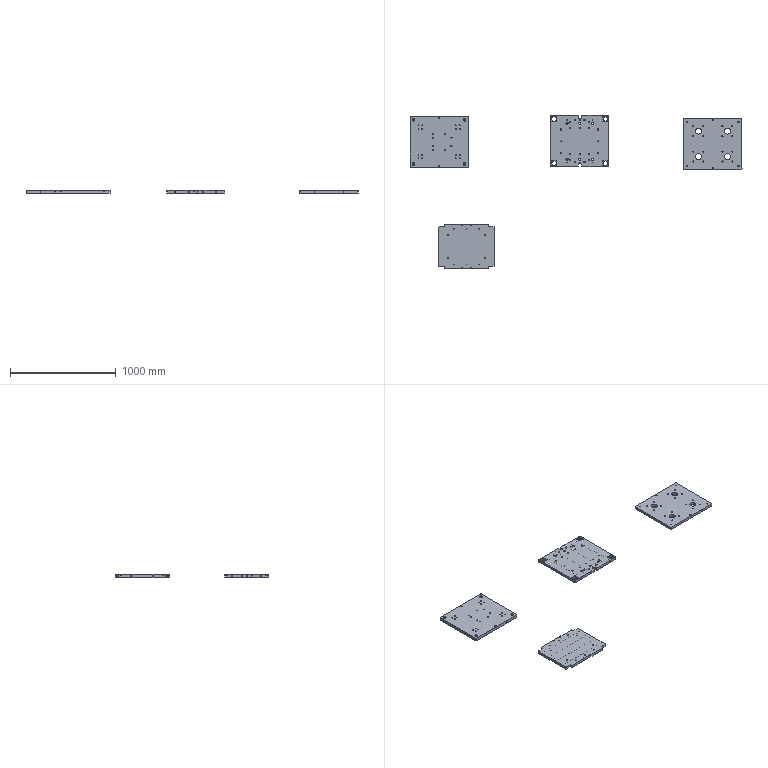NC program | Mastercam | posted with a generic post | part box 3140 x 1452 x 30 mm
Lines 1 to 2161 of 22248, first 1813 of 2161 lines:
%
O0000()
(MATERIAL - ALUMINUM MM - 2024)
( T16 | 16 FEM | H16 | XY STOCK TO LEAVE - .1 | Z STOCK TO LEAVE - .05 )
( T12 | 12 FEM | H12 | XY STOCK TO LEAVE - 0. | Z STOCK TO LEAVE - .05 )
( T7 | 4 CHM | H7 )
( T6 | 6 FEM | H6 | XY STOCK TO LEAVE - .05 | Z STOCK TO LEAVE - .15 )
( T15 | 5.2 DR | H15 | XY STOCK TO LEAVE - 0. | Z STOCK TO LEAVE - .15 )
( T3 | 10.5 DR | H3 )
( T19 | 9 DR | H19 )
N100 G21
N110 G0 G17 G40 G49 G80 G90
( ? )
N120 T16 M6
N130 G0 G90 G54 X-283.1 Y-255.5 A0. S6000 M3
N140 G43 H16 Z50. M8
N150 Z1.
N160 G1 Z-.499 F600.
N170 Y-237.5 F4000.
N180 Y237.5
N190 Y255.5
N200 Z-.998 F600.
N210 Y237.5 F4000.
N220 Y-237.5
N230 Y-255.5
N240 Z-1.497 F600.
N250 Y-237.5 F4000.
N260 Y237.5
N270 Y255.5
N280 Z-1.996 F600.
N290 Y237.5 F4000.
N300 Y-237.5
N310 Y-255.5
N320 Z-2.495 F600.
N330 Y-237.5 F4000.
N340 Y237.5
N350 Y255.5
N360 Z-2.994 F600.
N370 Y237.5 F4000.
N380 Y-237.5
N390 Y-255.5
N400 Z-3.493 F600.
N410 Y-237.5 F4000.
N420 Y237.5
N430 Y255.5
N440 Z-3.992 F600.
N450 Y237.5 F4000.
N460 Y-237.5
N470 Y-255.5
N480 Z-4.491 F600.
N490 Y-237.5 F4000.
N500 Y237.5
N510 Y255.5
N520 Z-4.99 F600.
N530 Y237.5 F4000.
N540 Y-237.5
N550 Y-255.5
N560 Z-5.489 F600.
N570 Y-237.5 F4000.
N580 Y237.5
N590 Y255.5
N600 Z-5.988 F600.
N610 Y237.5 F4000.
N620 Y-237.5
N630 Y-255.5
N640 Z-6.487 F600.
N650 Y-237.5 F4000.
N660 Y237.5
N670 Y255.5
N680 Z-6.986 F600.
N690 Y237.5 F4000.
N700 Y-237.5
N710 Y-255.5
N720 Z-7.485 F600.
N730 Y-237.5 F4000.
N740 Y237.5
N750 Y255.5
N760 Z-7.984 F600.
N770 Y237.5 F4000.
N780 Y-237.5
N790 Y-255.5
N800 Z-8.483 F600.
N810 Y-237.5 F4000.
N820 Y237.5
N830 Y255.5
N840 Z-8.982 F600.
N850 Y237.5 F4000.
N860 Y-237.5
N870 Y-255.5
N880 Z-9.481 F600.
N890 Y-237.5 F4000.
N900 Y237.5
N910 Y255.5
N920 Z-9.98 F600.
N930 Y237.5 F4000.
N940 Y-237.5
N950 Y-255.5
N960 Z-10.479 F600.
N970 Y-237.5 F4000.
N980 Y237.5
N990 Y255.5
N1000 Z-10.978 F600.
N1010 Y237.5 F4000.
N1020 Y-237.5
N1030 Y-255.5
N1040 Z-11.477 F600.
N1050 Y-237.5 F4000.
N1060 Y237.5
N1070 Y255.5
N1080 Z-11.976 F600.
N1090 Y237.5 F4000.
N1100 Y-237.5
N1110 Y-255.5
N1120 Z-12.475 F600.
N1130 Y-237.5 F4000.
N1140 Y237.5
N1150 Y255.5
N1160 Z-12.974 F600.
N1170 Y237.5 F4000.
N1180 Y-237.5
N1190 Y-255.5
N1200 Z-13.473 F600.
N1210 Y-237.5 F4000.
N1220 Y237.5
N1230 Y255.5
N1240 Z-13.972 F600.
N1250 Y237.5 F4000.
N1260 Y-237.5
N1270 Y-255.5
N1280 Z-14.471 F600.
N1290 Y-237.5 F4000.
N1300 Y237.5
N1310 Y255.5
N1320 Z-14.97 F600.
N1330 Y237.5 F4000.
N1340 Y-237.5
N1350 Y-255.5
N1360 Z-15.469 F600.
N1370 Y-237.5 F4000.
N1380 Y237.5
N1390 Y255.5
N1400 Z-15.968 F600.
N1410 Y237.5 F4000.
N1420 Y-237.5
N1430 Y-255.5
N1440 Z-16.467 F600.
N1450 Y-237.5 F4000.
N1460 Y237.5
N1470 Y255.5
N1480 Z-16.966 F600.
N1490 Y237.5 F4000.
N1500 Y-237.5
N1510 Y-255.5
N1520 Z-17.465 F600.
N1530 Y-237.5 F4000.
N1540 Y237.5
N1550 Y255.5
N1560 Z-17.964 F600.
N1570 Y237.5 F4000.
N1580 Y-237.5
N1590 Y-255.5
N1600 Z-18.463 F600.
N1610 Y-237.5 F4000.
N1620 Y237.5
N1630 Y255.5
N1640 Z-18.962 F600.
N1650 Y237.5 F4000.
N1660 Y-237.5
N1670 Y-255.5
N1680 Z-19.461 F600.
N1690 Y-237.5 F4000.
N1700 Y237.5
N1710 Y255.5
N1720 Z-19.96 F600.
N1730 Y237.5 F4000.
N1740 Y-237.5
N1750 Y-255.5
N1760 Z-20.459 F600.
N1770 Y-237.5 F4000.
N1780 Y237.5
N1790 Y255.5
N1800 Z-20.958 F600.
N1810 Y237.5 F4000.
N1820 Y-237.5
N1830 Y-255.5
N1840 Z-21.457 F600.
N1850 Y-237.5 F4000.
N1860 Y237.5
N1870 Y255.5
N1880 Z-21.956 F600.
N1890 Y237.5 F4000.
N1900 Y-237.5
N1910 Y-255.5
N1920 Z-22.455 F600.
N1930 Y-237.5 F4000.
N1940 Y237.5
N1950 Y255.5
N1960 Z-22.954 F600.
N1970 Y237.5 F4000.
N1980 Y-237.5
N1990 Y-255.5
N2000 Z-23.453 F600.
N2010 Y-237.5 F4000.
N2020 Y237.5
N2030 Y255.5
N2040 Z-23.952 F600.
N2050 Y237.5 F4000.
N2060 Y-237.5
N2070 Y-255.5
N2080 Z-24.451 F600.
N2090 Y-237.5 F4000.
N2100 Y237.5
N2110 Y255.5
N2120 Z-24.95 F600.
N2130 Y237.5 F4000.
N2140 Y-237.5
N2150 Y-255.5
N2160 G0 Z50.
N2170 X283.1 Y255.5
N2180 Z1.
N2190 G1 Z-.499 F600.
N2200 Y237.5 F4000.
N2210 Y-237.5
N2220 Y-255.5
N2230 Z-.998 F600.
N2240 Y-237.5 F4000.
N2250 Y237.5
N2260 Y255.5
N2270 Z-1.497 F600.
N2280 Y237.5 F4000.
N2290 Y-237.5
N2300 Y-255.5
N2310 Z-1.996 F600.
N2320 Y-237.5 F4000.
N2330 Y237.5
N2340 Y255.5
N2350 Z-2.495 F600.
N2360 Y237.5 F4000.
N2370 Y-237.5
N2380 Y-255.5
N2390 Z-2.994 F600.
N2400 Y-237.5 F4000.
N2410 Y237.5
N2420 Y255.5
N2430 Z-3.493 F600.
N2440 Y237.5 F4000.
N2450 Y-237.5
N2460 Y-255.5
N2470 Z-3.992 F600.
N2480 Y-237.5 F4000.
N2490 Y237.5
N2500 Y255.5
N2510 Z-4.491 F600.
N2520 Y237.5 F4000.
N2530 Y-237.5
N2540 Y-255.5
N2550 Z-4.99 F600.
N2560 Y-237.5 F4000.
N2570 Y237.5
N2580 Y255.5
N2590 Z-5.489 F600.
N2600 Y237.5 F4000.
N2610 Y-237.5
N2620 Y-255.5
N2630 Z-5.988 F600.
N2640 Y-237.5 F4000.
N2650 Y237.5
N2660 Y255.5
N2670 Z-6.487 F600.
N2680 Y237.5 F4000.
N2690 Y-237.5
N2700 Y-255.5
N2710 Z-6.986 F600.
N2720 Y-237.5 F4000.
N2730 Y237.5
N2740 Y255.5
N2750 Z-7.485 F600.
N2760 Y237.5 F4000.
N2770 Y-237.5
N2780 Y-255.5
N2790 Z-7.984 F600.
N2800 Y-237.5 F4000.
N2810 Y237.5
N2820 Y255.5
N2830 Z-8.483 F600.
N2840 Y237.5 F4000.
N2850 Y-237.5
N2860 Y-255.5
N2870 Z-8.982 F600.
N2880 Y-237.5 F4000.
N2890 Y237.5
N2900 Y255.5
N2910 Z-9.481 F600.
N2920 Y237.5 F4000.
N2930 Y-237.5
N2940 Y-255.5
N2950 Z-9.98 F600.
N2960 Y-237.5 F4000.
N2970 Y237.5
N2980 Y255.5
N2990 Z-10.479 F600.
N3000 Y237.5 F4000.
N3010 Y-237.5
N3020 Y-255.5
N3030 Z-10.978 F600.
N3040 Y-237.5 F4000.
N3050 Y237.5
N3060 Y255.5
N3070 Z-11.477 F600.
N3080 Y237.5 F4000.
N3090 Y-237.5
N3100 Y-255.5
N3110 Z-11.976 F600.
N3120 Y-237.5 F4000.
N3130 Y237.5
N3140 Y255.5
N3150 Z-12.475 F600.
N3160 Y237.5 F4000.
N3170 Y-237.5
N3180 Y-255.5
N3190 Z-12.974 F600.
N3200 Y-237.5 F4000.
N3210 Y237.5
N3220 Y255.5
N3230 Z-13.473 F600.
N3240 Y237.5 F4000.
N3250 Y-237.5
N3260 Y-255.5
N3270 Z-13.972 F600.
N3280 Y-237.5 F4000.
N3290 Y237.5
N3300 Y255.5
N3310 Z-14.471 F600.
N3320 Y237.5 F4000.
N3330 Y-237.5
N3340 Y-255.5
N3350 Z-14.97 F600.
N3360 Y-237.5 F4000.
N3370 Y237.5
N3380 Y255.5
N3390 Z-15.469 F600.
N3400 Y237.5 F4000.
N3410 Y-237.5
N3420 Y-255.5
N3430 Z-15.968 F600.
N3440 Y-237.5 F4000.
N3450 Y237.5
N3460 Y255.5
N3470 Z-16.467 F600.
N3480 Y237.5 F4000.
N3490 Y-237.5
N3500 Y-255.5
N3510 Z-16.966 F600.
N3520 Y-237.5 F4000.
N3530 Y237.5
N3540 Y255.5
N3550 Z-17.465 F600.
N3560 Y237.5 F4000.
N3570 Y-237.5
N3580 Y-255.5
N3590 Z-17.964 F600.
N3600 Y-237.5 F4000.
N3610 Y237.5
N3620 Y255.5
N3630 Z-18.463 F600.
N3640 Y237.5 F4000.
N3650 Y-237.5
N3660 Y-255.5
N3670 Z-18.962 F600.
N3680 Y-237.5 F4000.
N3690 Y237.5
N3700 Y255.5
N3710 Z-19.461 F600.
N3720 Y237.5 F4000.
N3730 Y-237.5
N3740 Y-255.5
N3750 Z-19.96 F600.
N3760 Y-237.5 F4000.
N3770 Y237.5
N3780 Y255.5
N3790 Z-20.459 F600.
N3800 Y237.5 F4000.
N3810 Y-237.5
N3820 Y-255.5
N3830 Z-20.958 F600.
N3840 Y-237.5 F4000.
N3850 Y237.5
N3860 Y255.5
N3870 Z-21.457 F600.
N3880 Y237.5 F4000.
N3890 Y-237.5
N3900 Y-255.5
N3910 Z-21.956 F600.
N3920 Y-237.5 F4000.
N3930 Y237.5
N3940 Y255.5
N3950 Z-22.455 F600.
N3960 Y237.5 F4000.
N3970 Y-237.5
N3980 Y-255.5
N3990 Z-22.954 F600.
N4000 Y-237.5 F4000.
N4010 Y237.5
N4020 Y255.5
N4030 Z-23.453 F600.
N4040 Y237.5 F4000.
N4050 Y-237.5
N4060 Y-255.5
N4070 Z-23.952 F600.
N4080 Y-237.5 F4000.
N4090 Y237.5
N4100 Y255.5
N4110 Z-24.451 F600.
N4120 Y237.5 F4000.
N4130 Y-237.5
N4140 Y-255.5
N4150 Z-24.95 F600.
N4160 Y-237.5 F4000.
N4170 Y237.5
N4180 Y255.5
N4190 G0 Z50.
N4200 M5
N4210 G91 G28 Z0. M9
N4220 A0.
N4230 M01
N4240 T12 M6
N4250 G0 G90 G17 G54 X-281. Y-255.5 A0. S6000 M3
N4260 G43 H12 Z50. M8
N4270 Z1.
N4280 G1 Z-12.475 F600.
N4290 Y-237.5 F1000.
N4300 Y237.5
N4310 Y255.5
N4320 G0 Z50.
N4330 Y-255.5
N4340 Z-11.475
N4350 G1 Z-24.95 F600.
N4360 Y-237.5 F1000.
N4370 Y237.5
N4380 Y255.5
N4390 G0 Z50.
N4400 X281.
N4410 Z1.
N4420 G1 Z-12.475 F600.
N4430 Y237.5 F1000.
N4440 Y-237.5
N4450 Y-255.5
N4460 G0 Z50.
N4470 Y255.5
N4480 Z-11.475
N4490 G1 Z-24.95 F600.
N4500 Y237.5 F1000.
N4510 Y-237.5
N4520 Y-255.5
N4530 G0 Z50.
N4540 M5
N4550 G91 G28 Z0. M9
N4560 A0.
N4570 M01
N4580 T7 M6
N4590 G0 G90 G17 G54 X-275.65 Y-242.5 A0. S6000 M3
N4600 G43 H7 Z50. M8
N4610 Z1.
N4620 G1 Z-.75 F600.
N4630 Y-237.5 F1000.
N4640 Y237.5
N4650 Y242.5
N4660 G0 Z50.
N4670 X275.65
N4680 Z1.
N4690 G1 Z-.75 F600.
N4700 Y237.5 F1000.
N4710 Y-237.5
N4720 Y-242.5
N4730 G0 Z50.
N4740 M5
N4750 G91 G28 Z0. M9
N4760 A0.
N4770 M01
( ?X )
M00
N4780 T16 M6
N4790 G0 G90 G17 G54 X-4. Y253.5 A0. S6000 M3
N4800 G43 H16 Z50. M8
N4810 Z1.
N4820 G1 Z-.693 F600.
N4830 Y237.5 F4000.
N4840 Y225.
N4850 G3 X0. Y221. I4. J0.
N4860 X4. Y225. I0. J4.
N4870 G1 Y237.5
N4880 Y253.5
N4890 Z-1.386 F600.
N4900 Y237.5 F4000.
N4910 Y225.
N4920 G2 X0. Y221. I-4. J0.
N4930 X-4. Y225. I0. J4.
N4940 G1 Y237.5
N4950 Y253.5
N4960 Z-2.079 F600.
N4970 Y237.5 F4000.
N4980 Y225.
N4990 G3 X0. Y221. I4. J0.
N5000 X4. Y225. I0. J4.
N5010 G1 Y237.5
N5020 Y253.5
N5030 Z-2.772 F600.
N5040 Y237.5 F4000.
N5050 Y225.
N5060 G2 X0. Y221. I-4. J0.
N5070 X-4. Y225. I0. J4.
N5080 G1 Y237.5
N5090 Y253.5
N5100 Z-3.465 F600.
N5110 Y237.5 F4000.
N5120 Y225.
N5130 G3 X0. Y221. I4. J0.
N5140 X4. Y225. I0. J4.
N5150 G1 Y237.5
N5160 Y253.5
N5170 Z-4.158 F600.
N5180 Y237.5 F4000.
N5190 Y225.
N5200 G2 X0. Y221. I-4. J0.
N5210 X-4. Y225. I0. J4.
N5220 G1 Y237.5
N5230 Y253.5
N5240 Z-4.851 F600.
N5250 Y237.5 F4000.
N5260 Y225.
N5270 G3 X0. Y221. I4. J0.
N5280 X4. Y225. I0. J4.
N5290 G1 Y237.5
N5300 Y253.5
N5310 Z-5.544 F600.
N5320 Y237.5 F4000.
N5330 Y225.
N5340 G2 X0. Y221. I-4. J0.
N5350 X-4. Y225. I0. J4.
N5360 G1 Y237.5
N5370 Y253.5
N5380 Z-6.237 F600.
N5390 Y237.5 F4000.
N5400 Y225.
N5410 G3 X0. Y221. I4. J0.
N5420 X4. Y225. I0. J4.
N5430 G1 Y237.5
N5440 Y253.5
N5450 Z-6.931 F600.
N5460 Y237.5 F4000.
N5470 Y225.
N5480 G2 X0. Y221. I-4. J0.
N5490 X-4. Y225. I0. J4.
N5500 G1 Y237.5
N5510 Y253.5
N5520 Z-7.624 F600.
N5530 Y237.5 F4000.
N5540 Y225.
N5550 G3 X0. Y221. I4. J0.
N5560 X4. Y225. I0. J4.
N5570 G1 Y237.5
N5580 Y253.5
N5590 Z-8.317 F600.
N5600 Y237.5 F4000.
N5610 Y225.
N5620 G2 X0. Y221. I-4. J0.
N5630 X-4. Y225. I0. J4.
N5640 G1 Y237.5
N5650 Y253.5
N5660 Z-9.01 F600.
N5670 Y237.5 F4000.
N5680 Y225.
N5690 G3 X0. Y221. I4. J0.
N5700 X4. Y225. I0. J4.
N5710 G1 Y237.5
N5720 Y253.5
N5730 Z-9.703 F600.
N5740 Y237.5 F4000.
N5750 Y225.
N5760 G2 X0. Y221. I-4. J0.
N5770 X-4. Y225. I0. J4.
N5780 G1 Y237.5
N5790 Y253.5
N5800 Z-10.396 F600.
N5810 Y237.5 F4000.
N5820 Y225.
N5830 G3 X0. Y221. I4. J0.
N5840 X4. Y225. I0. J4.
N5850 G1 Y237.5
N5860 Y253.5
N5870 Z-11.089 F600.
N5880 Y237.5 F4000.
N5890 Y225.
N5900 G2 X0. Y221. I-4. J0.
N5910 X-4. Y225. I0. J4.
N5920 G1 Y237.5
N5930 Y253.5
N5940 Z-11.782 F600.
N5950 Y237.5 F4000.
N5960 Y225.
N5970 G3 X0. Y221. I4. J0.
N5980 X4. Y225. I0. J4.
N5990 G1 Y237.5
N6000 Y253.5
N6010 Z-12.475 F600.
N6020 Y237.5 F4000.
N6030 Y225.
N6040 G2 X0. Y221. I-4. J0.
N6050 X-4. Y225. I0. J4.
N6060 G1 Y237.5
N6070 Y253.5
N6080 Z-13.168 F600.
N6090 Y237.5 F4000.
N6100 Y225.
N6110 G3 X0. Y221. I4. J0.
N6120 X4. Y225. I0. J4.
N6130 G1 Y237.5
N6140 Y253.5
N6150 Z-13.861 F600.
N6160 Y237.5 F4000.
N6170 Y225.
N6180 G2 X0. Y221. I-4. J0.
N6190 X-4. Y225. I0. J4.
N6200 G1 Y237.5
N6210 Y253.5
N6220 Z-14.554 F600.
N6230 Y237.5 F4000.
N6240 Y225.
N6250 G3 X0. Y221. I4. J0.
N6260 X4. Y225. I0. J4.
N6270 G1 Y237.5
N6280 Y253.5
N6290 Z-15.247 F600.
N6300 Y237.5 F4000.
N6310 Y225.
N6320 G2 X0. Y221. I-4. J0.
N6330 X-4. Y225. I0. J4.
N6340 G1 Y237.5
N6350 Y253.5
N6360 Z-15.94 F600.
N6370 Y237.5 F4000.
N6380 Y225.
N6390 G3 X0. Y221. I4. J0.
N6400 X4. Y225. I0. J4.
N6410 G1 Y237.5
N6420 Y253.5
N6430 Z-16.633 F600.
N6440 Y237.5 F4000.
N6450 Y225.
N6460 G2 X0. Y221. I-4. J0.
N6470 X-4. Y225. I0. J4.
N6480 G1 Y237.5
N6490 Y253.5
N6500 Z-17.326 F600.
N6510 Y237.5 F4000.
N6520 Y225.
N6530 G3 X0. Y221. I4. J0.
N6540 X4. Y225. I0. J4.
N6550 G1 Y237.5
N6560 Y253.5
N6570 Z-18.019 F600.
N6580 Y237.5 F4000.
N6590 Y225.
N6600 G2 X0. Y221. I-4. J0.
N6610 X-4. Y225. I0. J4.
N6620 G1 Y237.5
N6630 Y253.5
N6640 Z-18.712 F600.
N6650 Y237.5 F4000.
N6660 Y225.
N6670 G3 X0. Y221. I4. J0.
N6680 X4. Y225. I0. J4.
N6690 G1 Y237.5
N6700 Y253.5
N6710 Z-19.406 F600.
N6720 Y237.5 F4000.
N6730 Y225.
N6740 G2 X0. Y221. I-4. J0.
N6750 X-4. Y225. I0. J4.
N6760 G1 Y237.5
N6770 Y253.5
N6780 Z-20.099 F600.
N6790 Y237.5 F4000.
N6800 Y225.
N6810 G3 X0. Y221. I4. J0.
N6820 X4. Y225. I0. J4.
N6830 G1 Y237.5
N6840 Y253.5
N6850 Z-20.792 F600.
N6860 Y237.5 F4000.
N6870 Y225.
N6880 G2 X0. Y221. I-4. J0.
N6890 X-4. Y225. I0. J4.
N6900 G1 Y237.5
N6910 Y253.5
N6920 Z-21.485 F600.
N6930 Y237.5 F4000.
N6940 Y225.
N6950 G3 X0. Y221. I4. J0.
N6960 X4. Y225. I0. J4.
N6970 G1 Y237.5
N6980 Y253.5
N6990 Z-22.178 F600.
N7000 Y237.5 F4000.
N7010 Y225.
N7020 G2 X0. Y221. I-4. J0.
N7030 X-4. Y225. I0. J4.
N7040 G1 Y237.5
N7050 Y253.5
N7060 Z-22.871 F600.
N7070 Y237.5 F4000.
N7080 Y225.
N7090 G3 X0. Y221. I4. J0.
N7100 X4. Y225. I0. J4.
N7110 G1 Y237.5
N7120 Y253.5
N7130 Z-23.564 F600.
N7140 Y237.5 F4000.
N7150 Y225.
N7160 G2 X0. Y221. I-4. J0.
N7170 X-4. Y225. I0. J4.
N7180 G1 Y237.5
N7190 Y253.5
N7200 Z-24.257 F600.
N7210 Y237.5 F4000.
N7220 Y225.
N7230 G3 X0. Y221. I4. J0.
N7240 X4. Y225. I0. J4.
N7250 G1 Y237.5
N7260 Y253.5
N7270 Z-24.95 F600.
N7280 Y237.5 F4000.
N7290 Y225.
N7300 G2 X0. Y221. I-4. J0.
N7310 X-4. Y225. I0. J4.
N7320 G1 Y237.5
N7330 Y253.5
N7340 G0 Z50.
N7350 X4. Y-253.5
N7360 Z1.
N7370 G1 Z-.693 F600.
N7380 Y-237.5 F4000.
N7390 Y-225.
N7400 G3 X0. Y-221. I-4. J0.
N7410 X-4. Y-225. I0. J-4.
N7420 G1 Y-237.5
N7430 Y-253.5
N7440 Z-1.386 F600.
N7450 Y-237.5 F4000.
N7460 Y-225.
N7470 G2 X0. Y-221. I4. J0.
N7480 X4. Y-225. I0. J-4.
N7490 G1 Y-237.5
N7500 Y-253.5
N7510 Z-2.079 F600.
N7520 Y-237.5 F4000.
N7530 Y-225.
N7540 G3 X0. Y-221. I-4. J0.
N7550 X-4. Y-225. I0. J-4.
N7560 G1 Y-237.5
N7570 Y-253.5
N7580 Z-2.772 F600.
N7590 Y-237.5 F4000.
N7600 Y-225.
N7610 G2 X0. Y-221. I4. J0.
N7620 X4. Y-225. I0. J-4.
N7630 G1 Y-237.5
N7640 Y-253.5
N7650 Z-3.465 F600.
N7660 Y-237.5 F4000.
N7670 Y-225.
N7680 G3 X0. Y-221. I-4. J0.
N7690 X-4. Y-225. I0. J-4.
N7700 G1 Y-237.5
N7710 Y-253.5
N7720 Z-4.158 F600.
N7730 Y-237.5 F4000.
N7740 Y-225.
N7750 G2 X0. Y-221. I4. J0.
N7760 X4. Y-225. I0. J-4.
N7770 G1 Y-237.5
N7780 Y-253.5
N7790 Z-4.851 F600.
N7800 Y-237.5 F4000.
N7810 Y-225.
N7820 G3 X0. Y-221. I-4. J0.
N7830 X-4. Y-225. I0. J-4.
N7840 G1 Y-237.5
N7850 Y-253.5
N7860 Z-5.544 F600.
N7870 Y-237.5 F4000.
N7880 Y-225.
N7890 G2 X0. Y-221. I4. J0.
N7900 X4. Y-225. I0. J-4.
N7910 G1 Y-237.5
N7920 Y-253.5
N7930 Z-6.237 F600.
N7940 Y-237.5 F4000.
N7950 Y-225.
N7960 G3 X0. Y-221. I-4. J0.
N7970 X-4. Y-225. I0. J-4.
N7980 G1 Y-237.5
N7990 Y-253.5
N8000 Z-6.931 F600.
N8010 Y-237.5 F4000.
N8020 Y-225.
N8030 G2 X0. Y-221. I4. J0.
N8040 X4. Y-225. I0. J-4.
N8050 G1 Y-237.5
N8060 Y-253.5
N8070 Z-7.624 F600.
N8080 Y-237.5 F4000.
N8090 Y-225.
N8100 G3 X0. Y-221. I-4. J0.
N8110 X-4. Y-225. I0. J-4.
N8120 G1 Y-237.5
N8130 Y-253.5
N8140 Z-8.317 F600.
N8150 Y-237.5 F4000.
N8160 Y-225.
N8170 G2 X0. Y-221. I4. J0.
N8180 X4. Y-225. I0. J-4.
N8190 G1 Y-237.5
N8200 Y-253.5
N8210 Z-9.01 F600.
N8220 Y-237.5 F4000.
N8230 Y-225.
N8240 G3 X0. Y-221. I-4. J0.
N8250 X-4. Y-225. I0. J-4.
N8260 G1 Y-237.5
N8270 Y-253.5
N8280 Z-9.703 F600.
N8290 Y-237.5 F4000.
N8300 Y-225.
N8310 G2 X0. Y-221. I4. J0.
N8320 X4. Y-225. I0. J-4.
N8330 G1 Y-237.5
N8340 Y-253.5
N8350 Z-10.396 F600.
N8360 Y-237.5 F4000.
N8370 Y-225.
N8380 G3 X0. Y-221. I-4. J0.
N8390 X-4. Y-225. I0. J-4.
N8400 G1 Y-237.5
N8410 Y-253.5
N8420 Z-11.089 F600.
N8430 Y-237.5 F4000.
N8440 Y-225.
N8450 G2 X0. Y-221. I4. J0.
N8460 X4. Y-225. I0. J-4.
N8470 G1 Y-237.5
N8480 Y-253.5
N8490 Z-11.782 F600.
N8500 Y-237.5 F4000.
N8510 Y-225.
N8520 G3 X0. Y-221. I-4. J0.
N8530 X-4. Y-225. I0. J-4.
N8540 G1 Y-237.5
N8550 Y-253.5
N8560 Z-12.475 F600.
N8570 Y-237.5 F4000.
N8580 Y-225.
N8590 G2 X0. Y-221. I4. J0.
N8600 X4. Y-225. I0. J-4.
N8610 G1 Y-237.5
N8620 Y-253.5
N8630 Z-13.168 F600.
N8640 Y-237.5 F4000.
N8650 Y-225.
N8660 G3 X0. Y-221. I-4. J0.
N8670 X-4. Y-225. I0. J-4.
N8680 G1 Y-237.5
N8690 Y-253.5
N8700 Z-13.861 F600.
N8710 Y-237.5 F4000.
N8720 Y-225.
N8730 G2 X0. Y-221. I4. J0.
N8740 X4. Y-225. I0. J-4.
N8750 G1 Y-237.5
N8760 Y-253.5
N8770 Z-14.554 F600.
N8780 Y-237.5 F4000.
N8790 Y-225.
N8800 G3 X0. Y-221. I-4. J0.
N8810 X-4. Y-225. I0. J-4.
N8820 G1 Y-237.5
N8830 Y-253.5
N8840 Z-15.247 F600.
N8850 Y-237.5 F4000.
N8860 Y-225.
N8870 G2 X0. Y-221. I4. J0.
N8880 X4. Y-225. I0. J-4.
N8890 G1 Y-237.5
N8900 Y-253.5
N8910 Z-15.94 F600.
N8920 Y-237.5 F4000.
N8930 Y-225.
N8940 G3 X0. Y-221. I-4. J0.
N8950 X-4. Y-225. I0. J-4.
N8960 G1 Y-237.5
N8970 Y-253.5
N8980 Z-16.633 F600.
N8990 Y-237.5 F4000.
N9000 Y-225.
N9010 G2 X0. Y-221. I4. J0.
N9020 X4. Y-225. I0. J-4.
N9030 G1 Y-237.5
N9040 Y-253.5
N9050 Z-17.326 F600.
N9060 Y-237.5 F4000.
N9070 Y-225.
N9080 G3 X0. Y-221. I-4. J0.
N9090 X-4. Y-225. I0. J-4.
N9100 G1 Y-237.5
N9110 Y-253.5
N9120 Z-18.019 F600.
N9130 Y-237.5 F4000.
N9140 Y-225.
N9150 G2 X0. Y-221. I4. J0.
N9160 X4. Y-225. I0. J-4.
N9170 G1 Y-237.5
N9180 Y-253.5
N9190 Z-18.712 F600.
N9200 Y-237.5 F4000.
N9210 Y-225.
N9220 G3 X0. Y-221. I-4. J0.
N9230 X-4. Y-225. I0. J-4.
N9240 G1 Y-237.5
N9250 Y-253.5
N9260 Z-19.406 F600.
N9270 Y-237.5 F4000.
N9280 Y-225.
N9290 G2 X0. Y-221. I4. J0.
N9300 X4. Y-225. I0. J-4.
N9310 G1 Y-237.5
N9320 Y-253.5
N9330 Z-20.099 F600.
N9340 Y-237.5 F4000.
N9350 Y-225.
N9360 G3 X0. Y-221. I-4. J0.
N9370 X-4. Y-225. I0. J-4.
N9380 G1 Y-237.5
N9390 Y-253.5
N9400 Z-20.792 F600.
N9410 Y-237.5 F4000.
N9420 Y-225.
N9430 G2 X0. Y-221. I4. J0.
N9440 X4. Y-225. I0. J-4.
N9450 G1 Y-237.5
N9460 Y-253.5
N9470 Z-21.485 F600.
N9480 Y-237.5 F4000.
N9490 Y-225.
N9500 G3 X0. Y-221. I-4. J0.
N9510 X-4. Y-225. I0. J-4.
N9520 G1 Y-237.5
N9530 Y-253.5
N9540 Z-22.178 F600.
N9550 Y-237.5 F4000.
N9560 Y-225.
N9570 G2 X0. Y-221. I4. J0.
N9580 X4. Y-225. I0. J-4.
N9590 G1 Y-237.5
N9600 Y-253.5
N9610 Z-22.871 F600.
N9620 Y-237.5 F4000.
N9630 Y-225.
N9640 G3 X0. Y-221. I-4. J0.
N9650 X-4. Y-225. I0. J-4.
N9660 G1 Y-237.5
N9670 Y-253.5
N9680 Z-23.564 F600.
N9690 Y-237.5 F4000.
N9700 Y-225.
N9710 G2 X0. Y-221. I4. J0.
N9720 X4. Y-225. I0. J-4.
N9730 G1 Y-237.5
N9740 Y-253.5
N9750 Z-24.257 F600.
N9760 Y-237.5 F4000.
N9770 Y-225.
N9780 G3 X0. Y-221. I-4. J0.
N9790 X-4. Y-225. I0. J-4.
N9800 G1 Y-237.5
N9810 Y-253.5
N9820 Z-24.95 F600.
N9830 Y-237.5 F4000.
N9840 Y-225.
N9850 G2 X0. Y-221. I4. J0.
N9860 X4. Y-225. I0. J-4.
N9870 G1 Y-237.5
N9880 Y-253.5
N9890 G0 Z50.
N9900 X286.3 Y-235.9
N9910 Z1.
N9920 G1 Z-.693 F600.
N9930 X284.7 F4000.
N9940 G3 X283.1 Y-237.5 I0. J-1.6
N9950 G2 X270. Y-250.6 I-13.1 J0.
N9960 G1 X20.
N9970 G2 X6.9 Y-237.5 I0. J13.1
N9980 G1 Y-225.
N9990 G3 X0. Y-218.1 I-6.9 J0.
N100 X-6.9 Y-225. I0. J-6.9
N110 G1 Y-237.5
N120 G2 X-20. Y-250.6 I-13.1 J0.
N130 G1 X-270.
N140 G2 X-283.1 Y-237.5 I0. J13.1
N150 G3 X-284.7 Y-235.9 I-1.6 J0.
N160 G1 X-286.3
N170 Z-1.386 F600.
N180 X-284.7 F4000.
N190 G2 X-283.1 Y-237.5 I0. J-1.6
N200 G3 X-270. Y-250.6 I13.1 J0.
N210 G1 X-20.
N220 G3 X-6.9 Y-237.5 I0. J13.1
N230 G1 Y-225.
N240 G2 X0. Y-218.1 I6.9 J0.
N250 X6.9 Y-225. I0. J-6.9
N260 G1 Y-237.5
N270 G3 X20. Y-250.6 I13.1 J0.
N280 G1 X270.
N290 G3 X283.1 Y-237.5 I0. J13.1
N300 G2 X284.7 Y-235.9 I1.6 J0.
N310 G1 X286.3
N320 Z-2.079 F600.
N330 X284.7 F4000.
N340 G3 X283.1 Y-237.5 I0. J-1.6
N350 G2 X270. Y-250.6 I-13.1 J0.
N360 G1 X20.
N370 G2 X6.9 Y-237.5 I0. J13.1
N380 G1 Y-225.
N390 G3 X0. Y-218.1 I-6.9 J0.
N400 X-6.9 Y-225. I0. J-6.9
N410 G1 Y-237.5
N420 G2 X-20. Y-250.6 I-13.1 J0.
N430 G1 X-270.
N440 G2 X-283.1 Y-237.5 I0. J13.1
N450 G3 X-284.7 Y-235.9 I-1.6 J0.
N460 G1 X-286.3
N470 Z-2.772 F600.
N480 X-284.7 F4000.
N490 G2 X-283.1 Y-237.5 I0. J-1.6
N500 G3 X-270. Y-250.6 I13.1 J0.
N510 G1 X-20.
N520 G3 X-6.9 Y-237.5 I0. J13.1
N530 G1 Y-225.
N540 G2 X0. Y-218.1 I6.9 J0.
N550 X6.9 Y-225. I0. J-6.9
N560 G1 Y-237.5
N570 G3 X20. Y-250.6 I13.1 J0.
N580 G1 X270.
N590 G3 X283.1 Y-237.5 I0. J13.1
N600 G2 X284.7 Y-235.9 I1.6 J0.
N610 G1 X286.3
N620 Z-3.465 F600.
N630 X284.7 F4000.
N640 G3 X283.1 Y-237.5 I0. J-1.6
N650 G2 X270. Y-250.6 I-13.1 J0.
N660 G1 X20.
N670 G2 X6.9 Y-237.5 I0. J13.1
N680 G1 Y-225.
N690 G3 X0. Y-218.1 I-6.9 J0.
N700 X-6.9 Y-225. I0. J-6.9
N710 G1 Y-237.5
N720 G2 X-20. Y-250.6 I-13.1 J0.
N730 G1 X-270.
N740 G2 X-283.1 Y-237.5 I0. J13.1
N750 G3 X-284.7 Y-235.9 I-1.6 J0.
N760 G1 X-286.3
N770 Z-4.158 F600.
N780 X-284.7 F4000.
N790 G2 X-283.1 Y-237.5 I0. J-1.6
N800 G3 X-270. Y-250.6 I13.1 J0.
N810 G1 X-20.
N820 G3 X-6.9 Y-237.5 I0. J13.1
N830 G1 Y-225.
N840 G2 X0. Y-218.1 I6.9 J0.
N850 X6.9 Y-225. I0. J-6.9
N860 G1 Y-237.5
N870 G3 X20. Y-250.6 I13.1 J0.
N880 G1 X270.
N890 G3 X283.1 Y-237.5 I0. J13.1
N900 G2 X284.7 Y-235.9 I1.6 J0.
N910 G1 X286.3
N920 Z-4.851 F600.
N930 X284.7 F4000.
N940 G3 X283.1 Y-237.5 I0. J-1.6
N950 G2 X270. Y-250.6 I-13.1 J0.
N960 G1 X20.
N970 G2 X6.9 Y-237.5 I0. J13.1
N980 G1 Y-225.
N990 G3 X0. Y-218.1 I-6.9 J0.
N1000 X-6.9 Y-225. I0. J-6.9
N1010 G1 Y-237.5
N1020 G2 X-20. Y-250.6 I-13.1 J0.
N1030 G1 X-270.
N1040 G2 X-283.1 Y-237.5 I0. J13.1
N1050 G3 X-284.7 Y-235.9 I-1.6 J0.
N1060 G1 X-286.3
N1070 Z-5.544 F600.
N1080 X-284.7 F4000.
N1090 G2 X-283.1 Y-237.5 I0. J-1.6
N1100 G3 X-270. Y-250.6 I13.1 J0.
N1110 G1 X-20.
N1120 G3 X-6.9 Y-237.5 I0. J13.1
N1130 G1 Y-225.
N1140 G2 X0. Y-218.1 I6.9 J0.
N1150 X6.9 Y-225. I0. J-6.9
N1160 G1 Y-237.5
N1170 G3 X20. Y-250.6 I13.1 J0.
N1180 G1 X270.
N1190 G3 X283.1 Y-237.5 I0. J13.1
N1200 G2 X284.7 Y-235.9 I1.6 J0.
N1210 G1 X286.3
N1220 Z-6.237 F600.
N1230 X284.7 F4000.
N1240 G3 X283.1 Y-237.5 I0. J-1.6
N1250 G2 X270. Y-250.6 I-13.1 J0.
N1260 G1 X20.
N1270 G2 X6.9 Y-237.5 I0. J13.1
N1280 G1 Y-225.
N1290 G3 X0. Y-218.1 I-6.9 J0.
N1300 X-6.9 Y-225. I0. J-6.9
N1310 G1 Y-237.5
N1320 G2 X-20. Y-250.6 I-13.1 J0.
N1330 G1 X-270.
N1340 G2 X-283.1 Y-237.5 I0. J13.1
N1350 G3 X-284.7 Y-235.9 I-1.6 J0.
N1360 G1 X-286.3
N1370 Z-6.931 F600.
N1380 X-284.7 F4000.
N1390 G2 X-283.1 Y-237.5 I0. J-1.6
N1400 G3 X-270. Y-250.6 I13.1 J0.
N1410 G1 X-20.
N1420 G3 X-6.9 Y-237.5 I0. J13.1
N1430 G1 Y-225.
N1440 G2 X0. Y-218.1 I6.9 J0.
N1450 X6.9 Y-225. I0. J-6.9
N1460 G1 Y-237.5
N1470 G3 X20. Y-250.6 I13.1 J0.
N1480 G1 X270.
N1490 G3 X283.1 Y-237.5 I0. J13.1
N1500 G2 X284.7 Y-235.9 I1.6 J0.
N1510 G1 X286.3
N1520 Z-7.624 F600.
N1530 X284.7 F4000.
N1540 G3 X283.1 Y-237.5 I0. J-1.6
N1550 G2 X270. Y-250.6 I-13.1 J0.
N1560 G1 X20.
N1570 G2 X6.9 Y-237.5 I0. J13.1
N1580 G1 Y-225.
N1590 G3 X0. Y-218.1 I-6.9 J0.
N1600 X-6.9 Y-225. I0. J-6.9
N1610 G1 Y-237.5
N1620 G2 X-20. Y-250.6 I-13.1 J0.
N1630 G1 X-270.
N1640 G2 X-283.1 Y-237.5 I0. J13.1
N1650 G3 X-284.7 Y-235.9 I-1.6 J0.
N1660 G1 X-286.3
N1670 Z-8.317 F600.
N1680 X-284.7 F4000.
N1690 G2 X-283.1 Y-237.5 I0. J-1.6
N1700 G3 X-270. Y-250.6 I13.1 J0.
N1710 G1 X-20.
N1720 G3 X-6.9 Y-237.5 I0. J13.1
N1730 G1 Y-225.
N1740 G2 X0. Y-218.1 I6.9 J0.
N1750 X6.9 Y-225. I0. J-6.9
N1760 G1 Y-237.5
N1770 G3 X20. Y-250.6 I13.1 J0.
N1780 G1 X270.
N1790 G3 X283.1 Y-237.5 I0. J13.1
N1800 G2 X284.7 Y-235.9 I1.6 J0.
N1810 G1 X286.3
N1820 Z-9.01 F600.
N1830 X284.7 F4000.
N1840 G3 X283.1 Y-237.5 I0. J-1.6
N1850 G2 X270. Y-250.6 I-13.1 J0.
N1860 G1 X20.
N1870 G2 X6.9 Y-237.5 I0. J13.1
N1880 G1 Y-225.
N1890 G3 X0. Y-218.1 I-6.9 J0.
N1900 X-6.9 Y-225. I0. J-6.9
N1910 G1 Y-237.5
N1920 G2 X-20. Y-250.6 I-13.1 J0.
N1930 G1 X-270.
N1940 G2 X-283.1 Y-237.5 I0. J13.1
N1950 G3 X-284.7 Y-235.9 I-1.6 J0.
N1960 G1 X-286.3
N1970 Z-9.703 F600.
N1980 X-284.7 F4000.
N1990 G2 X-283.1 Y-237.5 I0. J-1.6
N2000 G3 X-270. Y-250.6 I13.1 J0.
N2010 G1 X-20.
N2020 G3 X-6.9 Y-237.5 I0. J13.1
N2030 G1 Y-225.
N2040 G2 X0. Y-218.1 I6.9 J0.
N2050 X6.9 Y-225. I0. J-6.9
N2060 G1 Y-237.5
N2070 G3 X20. Y-250.6 I13.1 J0.
N2080 G1 X270.
N2090 G3 X283.1 Y-237.5 I0. J13.1
N2100 G2 X284.7 Y-235.9 I1.6 J0.
N2110 G1 X286.3
N2120 Z-10.396 F600.
N2130 X284.7 F4000.
N2140 G3 X283.1 Y-237.5 I0. J-1.6
N2150 G2 X270. Y-250.6 I-13.1 J0.
N2160 G1 X20.
N2170 G2 X6.9 Y-237.5 I0. J13.1
N2180 G1 Y-225.
N2190 G3 X0. Y-218.1 I-6.9 J0.
N2200 X-6.9 Y-225. I0. J-6.9
N2210 G1 Y-237.5
N2220 G2 X-20. Y-250.6 I-13.1 J0.
N2230 G1 X-270.
N2240 G2 X-283.1 Y-237.5 I0. J13.1
N2250 G3 X-284.7 Y-235.9 I-1.6 J0.
N2260 G1 X-286.3
N2270 Z-11.089 F600.
N2280 X-284.7 F4000.
N2290 G2 X-283.1 Y-237.5 I0. J-1.6
N2300 G3 X-270. Y-250.6 I13.1 J0.
N2310 G1 X-20.
N2320 G3 X-6.9 Y-237.5 I0. J13.1
N2330 G1 Y-225.
N2340 G2 X0. Y-218.1 I6.9 J0.
N2350 X6.9 Y-225. I0. J-6.9
N2360 G1 Y-237.5
N2370 G3 X20. Y-250.6 I13.1 J0.
N2380 G1 X270.
N2390 G3 X283.1 Y-237.5 I0. J13.1
N2400 G2 X284.7 Y-235.9 I1.6 J0.
N2410 G1 X286.3
N2420 Z-11.782 F600.
N2430 X284.7 F4000.
N2440 G3 X283.1 Y-237.5 I0. J-1.6
N2450 G2 X270. Y-250.6 I-13.1 J0.
N2460 G1 X20.
N2470 G2 X6.9 Y-237.5 I0. J13.1
N2480 G1 Y-225.
N2490 G3 X0. Y-218.1 I-6.9 J0.
N2500 X-6.9 Y-225. I0. J-6.9
N2510 G1 Y-237.5
N2520 G2 X-20. Y-250.6 I-13.1 J0.
N2530 G1 X-270.
N2540 G2 X-283.1 Y-237.5 I0. J13.1
N2550 G3 X-284.7 Y-235.9 I-1.6 J0.
N2560 G1 X-286.3
N2570 Z-12.475 F600.
N2580 X-284.7 F4000.
N2590 G2 X-283.1 Y-237.5 I0. J-1.6
N2600 G3 X-270. Y-250.6 I13.1 J0.
N2610 G1 X-20.
N2620 G3 X-6.9 Y-237.5 I0. J13.1
N2630 G1 Y-225.
N2640 G2 X0. Y-218.1 I6.9 J0.
N2650 X6.9 Y-225. I0. J-6.9
N2660 G1 Y-237.5
N2670 G3 X20. Y-250.6 I13.1 J0.
N2680 G1 X270.
N2690 G3 X283.1 Y-237.5 I0. J13.1
N2700 G2 X284.7 Y-235.9 I1.6 J0.
N2710 G1 X286.3
N2720 Z-13.168 F600.
N2730 X284.7 F4000.
N2740 G3 X283.1 Y-237.5 I0. J-1.6
N2750 G2 X270. Y-250.6 I-13.1 J0.
N2760 G1 X20.
N2770 G2 X6.9 Y-237.5 I0. J13.1
N2780 G1 Y-225.
N2790 G3 X0. Y-218.1 I-6.9 J0.
N2800 X-6.9 Y-225. I0. J-6.9
N2810 G1 Y-237.5
N2820 G2 X-20. Y-250.6 I-13.1 J0.
N2830 G1 X-270.
N2840 G2 X-283.1 Y-237.5 I0. J13.1
N2850 G3 X-284.7 Y-235.9 I-1.6 J0.
N2860 G1 X-286.3
N2870 Z-13.861 F600.
N2880 X-284.7 F4000.
N2890 G2 X-283.1 Y-237.5 I0. J-1.6
N2900 G3 X-270. Y-250.6 I13.1 J0.
N2910 G1 X-20.
N2920 G3 X-6.9 Y-237.5 I0. J13.1
N2930 G1 Y-225.
N2940 G2 X0. Y-218.1 I6.9 J0.
N2950 X6.9 Y-225. I0. J-6.9
N2960 G1 Y-237.5
N2970 G3 X20. Y-250.6 I13.1 J0.
N2980 G1 X270.
N2990 G3 X283.1 Y-237.5 I0. J13.1
N3000 G2 X284.7 Y-235.9 I1.6 J0.
N3010 G1 X286.3
N3020 Z-14.554 F600.
N3030 X284.7 F4000.
N3040 G3 X283.1 Y-237.5 I0. J-1.6
N3050 G2 X270. Y-250.6 I-13.1 J0.
N3060 G1 X20.
N3070 G2 X6.9 Y-237.5 I0. J13.1
N3080 G1 Y-225.
N3090 G3 X0. Y-218.1 I-6.9 J0.
N3100 X-6.9 Y-225. I0. J-6.9
N3110 G1 Y-237.5
N3120 G2 X-20. Y-250.6 I-13.1 J0.
N3130 G1 X-270.
N3140 G2 X-283.1 Y-237.5 I0. J13.1
N3150 G3 X-284.7 Y-235.9 I-1.6 J0.
N3160 G1 X-286.3
N3170 Z-15.247 F600.
N3180 X-284.7 F4000.
N3190 G2 X-283.1 Y-237.5 I0. J-1.6
N3200 G3 X-270. Y-250.6 I13.1 J0.
N3210 G1 X-20.
N3220 G3 X-6.9 Y-237.5 I0. J13.1
N3230 G1 Y-225.
N3240 G2 X0. Y-218.1 I6.9 J0.
N3250 X6.9 Y-225. I0. J-6.9
N3260 G1 Y-237.5
N3270 G3 X20. Y-250.6 I13.1 J0.
N3280 G1 X270.
N3290 G3 X283.1 Y-237.5 I0. J13.1
N3300 G2 X284.7 Y-235.9 I1.6 J0.
N3310 G1 X286.3
N3320 Z-15.94 F600.
N3330 X284.7 F4000.
N3340 G3 X283.1 Y-237.5 I0. J-1.6
N3350 G2 X270. Y-250.6 I-13.1 J0.
N3360 G1 X20.
N3370 G2 X6.9 Y-237.5 I0. J13.1
N3380 G1 Y-225.
N3390 G3 X0. Y-218.1 I-6.9 J0.
N3400 X-6.9 Y-225. I0. J-6.9
N3410 G1 Y-237.5
N3420 G2 X-20. Y-250.6 I-13.1 J0.
N3430 G1 X-270.
N3440 G2 X-283.1 Y-237.5 I0. J13.1
N3450 G3 X-284.7 Y-235.9 I-1.6 J0.
N3460 G1 X-286.3
N3470 Z-16.633 F600.
N3480 X-284.7 F4000.
N3490 G2 X-283.1 Y-237.5 I0. J-1.6
N3500 G3 X-270. Y-250.6 I13.1 J0.
N3510 G1 X-20.
N3520 G3 X-6.9 Y-237.5 I0. J13.1
N3530 G1 Y-225.
N3540 G2 X0. Y-218.1 I6.9 J0.
N3550 X6.9 Y-225. I0. J-6.9
N3560 G1 Y-237.5
N3570 G3 X20. Y-250.6 I13.1 J0.
N3580 G1 X270.
N3590 G3 X283.1 Y-237.5 I0. J13.1
N3600 G2 X284.7 Y-235.9 I1.6 J0.
N3610 G1 X286.3
N3620 Z-17.326 F600.
N3630 X284.7 F4000.
N3640 G3 X283.1 Y-237.5 I0. J-1.6
N3650 G2 X270. Y-250.6 I-13.1 J0.
N3660 G1 X20.
N3670 G2 X6.9 Y-237.5 I0. J13.1
N3680 G1 Y-225.
N3690 G3 X0. Y-218.1 I-6.9 J0.
N3700 X-6.9 Y-225. I0. J-6.9
N3710 G1 Y-237.5
N3720 G2 X-20. Y-250.6 I-13.1 J0.
N3730 G1 X-270.
N3740 G2 X-283.1 Y-237.5 I0. J13.1
N3750 G3 X-284.7 Y-235.9 I-1.6 J0.
N3760 G1 X-286.3
N3770 Z-18.019 F600.
N3780 X-284.7 F4000.
N3790 G2 X-283.1 Y-237.5 I0. J-1.6
N3800 G3 X-270. Y-250.6 I13.1 J0.
N3810 G1 X-20.
N3820 G3 X-6.9 Y-237.5 I0. J13.1
N3830 G1 Y-225.
N3840 G2 X0. Y-218.1 I6.9 J0.
N3850 X6.9 Y-225. I0. J-6.9
N3860 G1 Y-237.5
N3870 G3 X20. Y-250.6 I13.1 J0.
N3880 G1 X270.
N3890 G3 X283.1 Y-237.5 I0. J13.1
N3900 G2 X284.7 Y-235.9 I1.6 J0.
N3910 G1 X286.3
N3920 Z-18.712 F600.
N3930 X284.7 F4000.
N3940 G3 X283.1 Y-237.5 I0. J-1.6
N3950 G2 X270. Y-250.6 I-13.1 J0.
N3960 G1 X20.
N3970 G2 X6.9 Y-237.5 I0. J13.1
N3980 G1 Y-225.
N3990 G3 X0. Y-218.1 I-6.9 J0.
N4000 X-6.9 Y-225. I0. J-6.9
N4010 G1 Y-237.5
N4020 G2 X-20. Y-250.6 I-13.1 J0.
N4030 G1 X-270.
N4040 G2 X-283.1 Y-237.5 I0. J13.1
N4050 G3 X-284.7 Y-235.9 I-1.6 J0.
N4060 G1 X-286.3
N4070 Z-19.406 F600.
N4080 X-284.7 F4000.
N4090 G2 X-283.1 Y-237.5 I0. J-1.6
N4100 G3 X-270. Y-250.6 I13.1 J0.
N4110 G1 X-20.
N4120 G3 X-6.9 Y-237.5 I0. J13.1
N4130 G1 Y-225.
N4140 G2 X0. Y-218.1 I6.9 J0.
N4150 X6.9 Y-225. I0. J-6.9
N4160 G1 Y-237.5
N4170 G3 X20. Y-250.6 I13.1 J0.
N4180 G1 X270.
N4190 G3 X283.1 Y-237.5 I0. J13.1
N4200 G2 X284.7 Y-235.9 I1.6 J0.
N4210 G1 X286.3
N4220 Z-20.099 F600.
N4230 X284.7 F4000.
N4240 G3 X283.1 Y-237.5 I0. J-1.6
N4250 G2 X270. Y-250.6 I-13.1 J0.
N4260 G1 X20.
N4270 G2 X6.9 Y-237.5 I0. J13.1
N4280 G1 Y-225.
N4290 G3 X0. Y-218.1 I-6.9 J0.
N4300 X-6.9 Y-225. I0. J-6.9
N4310 G1 Y-237.5
N4320 G2 X-20. Y-250.6 I-13.1 J0.
N4330 G1 X-270.
N4340 G2 X-283.1 Y-237.5 I0. J13.1
N4350 G3 X-284.7 Y-235.9 I-1.6 J0.
N4360 G1 X-286.3
N4370 Z-20.792 F600.
N4380 X-284.7 F4000.
N4390 G2 X-283.1 Y-237.5 I0. J-1.6
N4400 G3 X-270. Y-250.6 I13.1 J0.
N4410 G1 X-20.
N4420 G3 X-6.9 Y-237.5 I0. J13.1
N4430 G1 Y-225.
N4440 G2 X0. Y-218.1 I6.9 J0.
N4450 X6.9 Y-225. I0. J-6.9
N4460 G1 Y-237.5
N4470 G3 X20. Y-250.6 I13.1 J0.
N4480 G1 X270.
N4490 G3 X283.1 Y-237.5 I0. J13.1
N4500 G2 X284.7 Y-235.9 I1.6 J0.
N4510 G1 X286.3
N4520 Z-21.485 F600.
N4530 X284.7 F4000.
N4540 G3 X283.1 Y-237.5 I0. J-1.6
N4550 G2 X270. Y-250.6 I-13.1 J0.
N4560 G1 X20.
N4570 G2 X6.9 Y-237.5 I0. J13.1
N4580 G1 Y-225.
N4590 G3 X0. Y-218.1 I-6.9 J0.
N4600 X-6.9 Y-225. I0. J-6.9
N4610 G1 Y-237.5
N4620 G2 X-20. Y-250.6 I-13.1 J0.
N4630 G1 X-270.
N4640 G2 X-283.1 Y-237.5 I0. J13.1
N4650 G3 X-284.7 Y-235.9 I-1.6 J0.
N4660 G1 X-286.3
N4670 Z-22.178 F600.
N4680 X-284.7 F4000.
N4690 G2 X-283.1 Y-237.5 I0. J-1.6
N4700 G3 X-270. Y-250.6 I13.1 J0.
N4710 G1 X-20.
N4720 G3 X-6.9 Y-237.5 I0. J13.1
N4730 G1 Y-225.
N4740 G2 X0. Y-218.1 I6.9 J0.
N4750 X6.9 Y-225. I0. J-6.9
N4760 G1 Y-237.5
N4770 G3 X20. Y-250.6 I13.1 J0.
N4780 G1 X270.
N4790 G3 X283.1 Y-237.5 I0. J13.1
N4800 G2 X284.7 Y-235.9 I1.6 J0.
N4810 G1 X286.3
N4820 Z-22.871 F600.
N4830 X284.7 F4000.
N4840 G3 X283.1 Y-237.5 I0. J-1.6
N4850 G2 X270. Y-250.6 I-13.1 J0.
N4860 G1 X20.
N4870 G2 X6.9 Y-237.5 I0. J13.1
N4880 G1 Y-225.
N4890 G3 X0. Y-218.1 I-6.9 J0.
N4900 X-6.9 Y-225. I0. J-6.9
N4910 G1 Y-237.5
N4920 G2 X-20. Y-250.6 I-13.1 J0.
N4930 G1 X-270.
N4940 G2 X-283.1 Y-237.5 I0. J13.1
N4950 G3 X-284.7 Y-235.9 I-1.6 J0.
N4960 G1 X-286.3
N4970 Z-23.564 F600.
N4980 X-284.7 F4000.
N4990 G2 X-283.1 Y-237.5 I0. J-1.6
N5000 G3 X-270. Y-250.6 I13.1 J0.
N5010 G1 X-20.
N5020 G3 X-6.9 Y-237.5 I0. J13.1
N5030 G1 Y-225.
N5040 G2 X0. Y-218.1 I6.9 J0.
N5050 X6.9 Y-225. I0. J-6.9
N5060 G1 Y-237.5
N5070 G3 X20. Y-250.6 I13.1 J0.
N5080 G1 X270.
N5090 G3 X283.1 Y-237.5 I0. J13.1
N5100 G2 X284.7 Y-235.9 I1.6 J0.
N5110 G1 X286.3
N5120 Z-24.257 F600.
N5130 X284.7 F4000.
N5140 G3 X283.1 Y-237.5 I0. J-1.6
N5150 G2 X270. Y-250.6 I-13.1 J0.
N5160 G1 X20.
N5170 G2 X6.9 Y-237.5 I0. J13.1
N5180 G1 Y-225.
N5190 G3 X0. Y-218.1 I-6.9 J0.
N5200 X-6.9 Y-225. I0. J-6.9
N5210 G1 Y-237.5
N5220 G2 X-20. Y-250.6 I-13.1 J0.
N5230 G1 X-270.
N5240 G2 X-283.1 Y-237.5 I0. J13.1
N5250 G3 X-284.7 Y-235.9 I-1.6 J0.
N5260 G1 X-286.3
N5270 Z-24.95 F600.
N5280 X-284.7 F4000.
N5290 G2 X-283.1 Y-237.5 I0. J-1.6
N5300 G3 X-270. Y-250.6 I13.1 J0.
N5310 G1 X-20.
N5320 G3 X-6.9 Y-237.5 I0. J13.1
N5330 G1 Y-225.
N5340 G2 X0. Y-218.1 I6.9 J0.
N5350 X6.9 Y-225. I0. J-6.9
N5360 G1 Y-237.5
N5370 G3 X20. Y-250.6 I13.1 J0.
N5380 G1 X270.
N5390 G3 X283.1 Y-237.5 I0. J13.1
N5400 G2 X284.7 Y-235.9 I1.6 J0.
N5410 G1 X286.3
N5420 G0 Z50.
N5430 X-286.3 Y235.9
N5440 Z1.
N5450 G1 Z-.693 F600.
N5460 X-284.7 F4000.
N5470 G3 X-283.1 Y237.5 I0. J1.6
N5480 G2 X-270. Y250.6 I13.1 J0.
N5490 G1 X-20.
N5500 G2 X-6.9 Y237.5 I0. J-13.1
N5510 G1 Y225.
N5520 G3 X0. Y218.1 I6.9 J0.
N5530 X6.9 Y225. I0. J6.9
N5540 G1 Y237.5
N5550 G2 X20. Y250.6 I13.1 J0.
N5560 G1 X270.
N5570 G2 X283.1 Y237.5 I0. J-13.1
N5580 G3 X284.7 Y235.9 I1.6 J0.
N5590 G1 X286.3
N5600 Z-1.386 F600.
N5610 X284.7 F4000.
N5620 G2 X283.1 Y237.5 I0. J1.6
N5630 G3 X270. Y250.6 I-13.1 J0.
N5640 G1 X20.
N5650 G3 X6.9 Y237.5 I0. J-13.1
N5660 G1 Y225.
N5670 G2 X0. Y218.1 I-6.9 J0.
N5680 X-6.9 Y225. I0. J6.9
N5690 G1 Y237.5
N5700 G3 X-20. Y250.6 I-13.1 J0.
N5710 G1 X-270.
N5720 G3 X-283.1 Y237.5 I0. J-13.1
N5730 G2 X-284.7 Y235.9 I-1.6 J0.
N5740 G1 X-286.3
N5750 Z-2.079 F600.
N5760 X-284.7 F4000.
N5770 G3 X-283.1 Y237.5 I0. J1.6
N5780 G2 X-270. Y250.6 I13.1 J0.
N5790 G1 X-20.
N5800 G2 X-6.9 Y237.5 I0. J-13.1
N5810 G1 Y225.
N5820 G3 X0. Y218.1 I6.9 J0.
N5830 X6.9 Y225. I0. J6.9
N5840 G1 Y237.5
N5850 G2 X20. Y250.6 I13.1 J0.
N5860 G1 X270.
N5870 G2 X283.1 Y237.5 I0. J-13.1
N5880 G3 X284.7 Y235.9 I1.6 J0.
N5890 G1 X286.3
N5900 Z-2.772 F600.
N5910 X284.7 F4000.
N5920 G2 X283.1 Y237.5 I0. J1.6
N5930 G3 X270. Y250.6 I-13.1 J0.
N5940 G1 X20.
N5950 G3 X6.9 Y237.5 I0. J-13.1
N5960 G1 Y225.
N5970 G2 X0. Y218.1 I-6.9 J0.
N5980 X-6.9 Y225. I0. J6.9
N5990 G1 Y237.5
N6000 G3 X-20. Y250.6 I-13.1 J0.
N6010 G1 X-270.
N6020 G3 X-283.1 Y237.5 I0. J-13.1
N6030 G2 X-284.7 Y235.9 I-1.6 J0.
N6040 G1 X-286.3
N6050 Z-3.465 F600.
N6060 X-284.7 F4000.
N6070 G3 X-283.1 Y237.5 I0. J1.6
N6080 G2 X-270. Y250.6 I13.1 J0.
N6090 G1 X-20.
N6100 G2 X-6.9 Y237.5 I0. J-13.1
N6110 G1 Y225.
N6120 G3 X0. Y218.1 I6.9 J0.
N6130 X6.9 Y225. I0. J6.9
N6140 G1 Y237.5
N6150 G2 X20. Y250.6 I13.1 J0.
N6160 G1 X270.
N6170 G2 X283.1 Y237.5 I0. J-13.1
N6180 G3 X284.7 Y235.9 I1.6 J0.
N6190 G1 X286.3
N6200 Z-4.158 F600.
N6210 X284.7 F4000.
N6220 G2 X283.1 Y237.5 I0. J1.6
N6230 G3 X270. Y250.6 I-13.1 J0.
N6240 G1 X20.
N6250 G3 X6.9 Y237.5 I0. J-13.1
N6260 G1 Y225.
N6270 G2 X0. Y218.1 I-6.9 J0.
N6280 X-6.9 Y225. I0. J6.9
N6290 G1 Y237.5
N6300 G3 X-20. Y250.6 I-13.1 J0.
N6310 G1 X-270.
N6320 G3 X-283.1 Y237.5 I0. J-13.1
N6330 G2 X-284.7 Y235.9 I-1.6 J0.
N6340 G1 X-286.3
N6350 Z-4.851 F600.
N6360 X-284.7 F4000.
N6370 G3 X-283.1 Y237.5 I0. J1.6
N6380 G2 X-270. Y250.6 I13.1 J0.
N6390 G1 X-20.
N6400 G2 X-6.9 Y237.5 I0. J-13.1
N6410 G1 Y225.
N6420 G3 X0. Y218.1 I6.9 J0.
N6430 X6.9 Y225. I0. J6.9
N6440 G1 Y237.5
N6450 G2 X20. Y250.6 I13.1 J0.
N6460 G1 X270.
N6470 G2 X283.1 Y237.5 I0. J-13.1
N6480 G3 X284.7 Y235.9 I1.6 J0.
N6490 G1 X286.3
N6500 Z-5.544 F600.
N6510 X284.7 F4000.
N6520 G2 X283.1 Y237.5 I0. J1.6
N6530 G3 X270. Y250.6 I-13.1 J0.
N6540 G1 X20.
N6550 G3 X6.9 Y237.5 I0. J-13.1
N6560 G1 Y225.
N6570 G2 X0. Y218.1 I-6.9 J0.
N6580 X-6.9 Y225. I0. J6.9
N6590 G1 Y237.5
N6600 G3 X-20. Y250.6 I-13.1 J0.
N6610 G1 X-270.
N6620 G3 X-283.1 Y237.5 I0. J-13.1
N6630 G2 X-284.7 Y235.9 I-1.6 J0.
N6640 G1 X-286.3
N6650 Z-6.237 F600.
N6660 X-284.7 F4000.
N6670 G3 X-283.1 Y237.5 I0. J1.6
N6680 G2 X-270. Y250.6 I13.1 J0.
N6690 G1 X-20.
N6700 G2 X-6.9 Y237.5 I0. J-13.1
N6710 G1 Y225.
N6720 G3 X0. Y218.1 I6.9 J0.
N6730 X6.9 Y225. I0. J6.9
N6740 G1 Y237.5
N6750 G2 X20. Y250.6 I13.1 J0.
N6760 G1 X270.
N6770 G2 X283.1 Y237.5 I0. J-13.1
N6780 G3 X284.7 Y235.9 I1.6 J0.
N6790 G1 X286.3
N6800 Z-6.931 F600.
N6810 X284.7 F4000.
N6820 G2 X283.1 Y237.5 I0. J1.6
N6830 G3 X270. Y250.6 I-13.1 J0.
N6840 G1 X20.
N6850 G3 X6.9 Y237.5 I0. J-13.1
N6860 G1 Y225.
N6870 G2 X0. Y218.1 I-6.9 J0.
N6880 X-6.9 Y225. I0. J6.9
N6890 G1 Y237.5
N6900 G3 X-20. Y250.6 I-13.1 J0.
N6910 G1 X-270.
N6920 G3 X-283.1 Y237.5 I0. J-13.1
N6930 G2 X-284.7 Y235.9 I-1.6 J0.
N6940 G1 X-286.3
N6950 Z-7.624 F600.
N6960 X-284.7 F4000.
N6970 G3 X-283.1 Y237.5 I0. J1.6
N6980 G2 X-270. Y250.6 I13.1 J0.
N6990 G1 X-20.
N7000 G2 X-6.9 Y237.5 I0. J-13.1
N7010 G1 Y225.
N7020 G3 X0. Y218.1 I6.9 J0.
N7030 X6.9 Y225. I0. J6.9
N7040 G1 Y237.5
N7050 G2 X20. Y250.6 I13.1 J0.
N7060 G1 X270.
N7070 G2 X283.1 Y237.5 I0. J-13.1
N7080 G3 X284.7 Y235.9 I1.6 J0.
N7090 G1 X286.3
N7100 Z-8.317 F600.
N7110 X284.7 F4000.
N7120 G2 X283.1 Y237.5 I0. J1.6
N7130 G3 X270. Y250.6 I-13.1 J0.
N7140 G1 X20.
N7150 G3 X6.9 Y237.5 I0. J-13.1
N7160 G1 Y225.
N7170 G2 X0. Y218.1 I-6.9 J0.
N7180 X-6.9 Y225. I0. J6.9
N7190 G1 Y237.5
N7200 G3 X-20. Y250.6 I-13.1 J0.
N7210 G1 X-270.
N7220 G3 X-283.1 Y237.5 I0. J-13.1
N7230 G2 X-284.7 Y235.9 I-1.6 J0.
N7240 G1 X-286.3
N7250 Z-9.01 F600.
N7260 X-284.7 F4000.
N7270 G3 X-283.1 Y237.5 I0. J1.6
N7280 G2 X-270. Y250.6 I13.1 J0.
N7290 G1 X-20.
N7300 G2 X-6.9 Y237.5 I0. J-13.1
N7310 G1 Y225.
N7320 G3 X0. Y218.1 I6.9 J0.
N7330 X6.9 Y225. I0. J6.9
N7340 G1 Y237.5
N7350 G2 X20. Y250.6 I13.1 J0.
N7360 G1 X270.
N7370 G2 X283.1 Y237.5 I0. J-13.1
N7380 G3 X284.7 Y235.9 I1.6 J0.
N7390 G1 X286.3
N7400 Z-9.703 F600.
N7410 X284.7 F4000.
N7420 G2 X283.1 Y237.5 I0. J1.6
N7430 G3 X270. Y250.6 I-13.1 J0.
N7440 G1 X20.
N7450 G3 X6.9 Y237.5 I0. J-13.1
N7460 G1 Y225.
N7470 G2 X0. Y218.1 I-6.9 J0.
N7480 X-6.9 Y225. I0. J6.9
N7490 G1 Y237.5
N7500 G3 X-20. Y250.6 I-13.1 J0.
N7510 G1 X-270.
N7520 G3 X-283.1 Y237.5 I0. J-13.1
N7530 G2 X-284.7 Y235.9 I-1.6 J0.
N7540 G1 X-286.3
N7550 Z-10.396 F600.
N7560 X-284.7 F4000.
N7570 G3 X-283.1 Y237.5 I0. J1.6
N7580 G2 X-270. Y250.6 I13.1 J0.
N7590 G1 X-20.
N7600 G2 X-6.9 Y237.5 I0. J-13.1
N7610 G1 Y225.
N7620 G3 X0. Y218.1 I6.9 J0.
N7630 X6.9 Y225. I0. J6.9
N7640 G1 Y237.5
N7650 G2 X20. Y250.6 I13.1 J0.
N7660 G1 X270.
N7670 G2 X283.1 Y237.5 I0. J-13.1
N7680 G3 X284.7 Y235.9 I1.6 J0.
N7690 G1 X286.3
N7700 Z-11.089 F600.
N7710 X284.7 F4000.
N7720 G2 X283.1 Y237.5 I0. J1.6
N7730 G3 X270. Y250.6 I-13.1 J0.
N7740 G1 X20.
N7750 G3 X6.9 Y237.5 I0. J-13.1
N7760 G1 Y225.
N7770 G2 X0. Y218.1 I-6.9 J0.
N7780 X-6.9 Y225. I0. J6.9
N7790 G1 Y237.5
N7800 G3 X-20. Y250.6 I-13.1 J0.
N7810 G1 X-270.
N7820 G3 X-283.1 Y237.5 I0. J-13.1
N7830 G2 X-284.7 Y235.9 I-1.6 J0.
N7840 G1 X-286.3
N7850 Z-11.782 F600.
N7860 X-284.7 F4000.
N7870 G3 X-283.1 Y237.5 I0. J1.6
N7880 G2 X-270. Y250.6 I13.1 J0.
N7890 G1 X-20.
N7900 G2 X-6.9 Y237.5 I0. J-13.1
N7910 G1 Y225.
N7920 G3 X0. Y218.1 I6.9 J0.
N7930 X6.9 Y225. I0. J6.9
N7940 G1 Y237.5
N7950 G2 X20. Y250.6 I13.1 J0.
N7960 G1 X270.
N7970 G2 X283.1 Y237.5 I0. J-13.1
N7980 G3 X284.7 Y235.9 I1.6 J0.
N7990 G1 X286.3
N8000 Z-12.475 F600.
N8010 X284.7 F4000.
N8020 G2 X283.1 Y237.5 I0. J1.6
N8030 G3 X270. Y250.6 I-13.1 J0.
N8040 G1 X20.
N8050 G3 X6.9 Y237.5 I0. J-13.1
N8060 G1 Y225.
N8070 G2 X0. Y218.1 I-6.9 J0.
N8080 X-6.9 Y225. I0. J6.9
N8090 G1 Y237.5
N8100 G3 X-20. Y250.6 I-13.1 J0.
N8110 G1 X-270.
N8120 G3 X-283.1 Y237.5 I0. J-13.1
N8130 G2 X-284.7 Y235.9 I-1.6 J0.
N8140 G1 X-286.3
N8150 Z-13.168 F600.
N8160 X-284.7 F4000.
N8170 G3 X-283.1 Y237.5 I0. J1.6
N8180 G2 X-270. Y250.6 I13.1 J0.
N8190 G1 X-20.